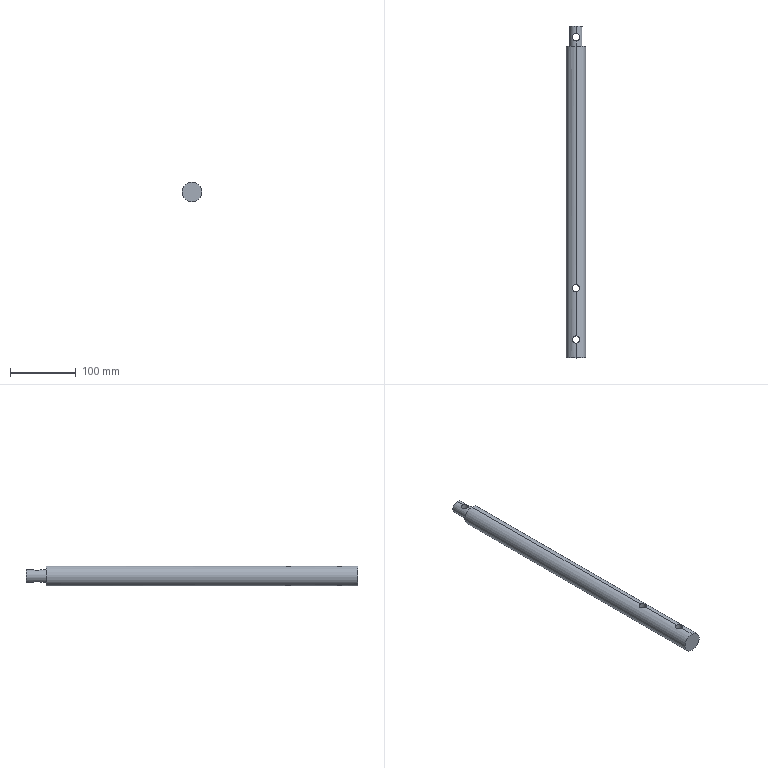Part | SolidWorks | features ICE 3, MoveFace 3, Extrusion 1 | 1 solid | 13 faces | box 30 x 504 x 30 mm | volume 335802 mm3 | cylinder 10 | plane 3 | commonest cylinder face diameters 11 x6 19 x2 30 x2
STEP:
#1=CARTESIAN_POINT('',(-5.5,288.,-13.955));
#2=VERTEX_POINT('',#1);
#3=CARTESIAN_POINT('',(0.,282.5,-15.));
#4=VERTEX_POINT('',#3);
#5=CARTESIAN_POINT('',(-5.5,288.,-13.955));
#6=CARTESIAN_POINT('',(-5.5,287.638,-13.955));
#7=CARTESIAN_POINT('',(-5.463,287.27,-13.97));
#8=CARTESIAN_POINT('',(-5.321,286.562,-14.025));
#9=CARTESIAN_POINT('',(-5.216,286.218,-14.065));
#10=CARTESIAN_POINT('',(-4.936,285.548,-14.165));
#11=CARTESIAN_POINT('',(-4.766,285.232,-14.224));
#12=CARTESIAN_POINT('',(-4.369,284.64,-14.351));
#13=CARTESIAN_POINT('',(-4.139,284.36,-14.42));
#14=CARTESIAN_POINT('',(-3.634,283.856,-14.555));
#15=CARTESIAN_POINT('',(-3.36,283.631,-14.622));
#16=CARTESIAN_POINT('',(-2.765,283.232,-14.746));
#17=CARTESIAN_POINT('',(-2.444,283.06,-14.803));
#18=CARTESIAN_POINT('',(-1.783,282.785,-14.897));
#19=CARTESIAN_POINT('',(-1.439,282.679,-14.935));
#20=CARTESIAN_POINT('',(-0.9036,282.572,-14.974));
#21=CARTESIAN_POINT('',(-0.7221,282.545,-14.984));
#22=CARTESIAN_POINT('',(-0.3611,282.509,-14.997));
#23=CARTESIAN_POINT('',(-0.1806,282.5,-15.));
#24=CARTESIAN_POINT('',(0.,282.5,-15.));
#25=B_SPLINE_CURVE_WITH_KNOTS('',3,(#5,#6,#7,#8,#9,#10,#11,#12,#13,#14,#15,#16,#17,#18,#19,#20,#21,#22,#23,#24),.UNSPECIFIED.,.F.,.F.,(4,2,2,2,2,2,2,2,2,4),(0.008677,0.009761,0.01084,0.01193,0.01301,0.0141,0.01518,0.01626,0.01681,0.01735),.UNSPECIFIED.);
#26=EDGE_CURVE('',#2,#4,#25,.T.);
#27=ORIENTED_EDGE('',*,*,#26,.F.);
#28=CARTESIAN_POINT('',(-5.5,288.,13.955));
#29=VERTEX_POINT('',#28);
#30=CARTESIAN_POINT('',(-5.5,288.,-215.));
#31=DIRECTION('',(0.,0.,1.));
#32=VECTOR('',#31,1000.);
#33=LINE('',#30,#32);
#34=EDGE_CURVE('',#2,#29,#33,.T.);
#35=ORIENTED_EDGE('',*,*,#34,.T.);
#36=CARTESIAN_POINT('',(0.,282.5,15.));
#37=VERTEX_POINT('',#36);
#38=CARTESIAN_POINT('',(0.,282.5,15.));
#39=CARTESIAN_POINT('',(-0.3624,282.5,15.));
#40=CARTESIAN_POINT('',(-0.7302,282.537,14.986));
#41=CARTESIAN_POINT('',(-1.438,282.679,14.935));
#42=CARTESIAN_POINT('',(-1.783,282.784,14.898));
#43=CARTESIAN_POINT('',(-2.453,283.064,14.802));
#44=CARTESIAN_POINT('',(-2.769,283.234,14.745));
#45=CARTESIAN_POINT('',(-3.361,283.632,14.622));
#46=CARTESIAN_POINT('',(-3.641,283.862,14.554));
#47=CARTESIAN_POINT('',(-4.145,284.368,14.418));
#48=CARTESIAN_POINT('',(-4.371,284.642,14.351));
#49=CARTESIAN_POINT('',(-4.768,285.236,14.223));
#50=CARTESIAN_POINT('',(-4.941,285.557,14.164));
#51=CARTESIAN_POINT('',(-5.216,286.218,14.065));
#52=CARTESIAN_POINT('',(-5.321,286.561,14.025));
#53=CARTESIAN_POINT('',(-5.428,287.096,13.983));
#54=CARTESIAN_POINT('',(-5.455,287.278,13.973));
#55=CARTESIAN_POINT('',(-5.491,287.639,13.959));
#56=CARTESIAN_POINT('',(-5.5,287.819,13.955));
#57=CARTESIAN_POINT('',(-5.5,288.,13.955));
#58=B_SPLINE_CURVE_WITH_KNOTS('',3,(#38,#39,#40,#41,#42,#43,#44,#45,#46,#47,#48,#49,#50,#51,#52,#53,#54,#55,#56,#57),.UNSPECIFIED.,.F.,.F.,(4,2,2,2,2,2,2,2,2,4),(0.008676,0.00976,0.01084,0.01193,0.01301,0.0141,0.01518,0.01626,0.01681,0.01735),.UNSPECIFIED.);
#59=EDGE_CURVE('',#37,#29,#58,.T.);
#60=ORIENTED_EDGE('',*,*,#59,.F.);
#61=CARTESIAN_POINT('',(5.5,288.,13.955));
#62=VERTEX_POINT('',#61);
#63=CARTESIAN_POINT('',(5.5,288.,13.955));
#64=CARTESIAN_POINT('',(5.5,287.633,13.955));
#65=CARTESIAN_POINT('',(5.464,287.273,13.97));
#66=CARTESIAN_POINT('',(5.322,286.565,14.024));
#67=CARTESIAN_POINT('',(5.215,286.214,14.065));
#68=CARTESIAN_POINT('',(4.937,285.55,14.165));
#69=CARTESIAN_POINT('',(4.768,285.235,14.224));
#70=CARTESIAN_POINT('',(4.469,284.789,14.319));
#71=CARTESIAN_POINT('',(4.361,284.644,14.353));
#72=CARTESIAN_POINT('',(4.133,284.367,14.42));
#73=CARTESIAN_POINT('',(4.013,284.235,14.454));
#74=CARTESIAN_POINT('',(3.636,283.858,14.555));
#75=CARTESIAN_POINT('',(3.361,283.631,14.622));
#76=CARTESIAN_POINT('',(2.761,283.229,14.747));
#77=CARTESIAN_POINT('',(2.445,283.061,14.803));
#78=CARTESIAN_POINT('',(1.949,282.854,14.874));
#79=CARTESIAN_POINT('',(1.78,282.793,14.895));
#80=CARTESIAN_POINT('',(1.434,282.687,14.932));
#81=CARTESIAN_POINT('',(1.256,282.642,14.948));
#82=CARTESIAN_POINT('',(0.7219,282.536,14.987));
#83=CARTESIAN_POINT('',(0.3626,282.5,15.));
#84=CARTESIAN_POINT('',(0.,282.5,15.));
#85=B_SPLINE_CURVE_WITH_KNOTS('',3,(#63,#64,#65,#66,#67,#68,#69,#70,#71,#72,#73,#74,#75,#76,#77,#78,#79,#80,#81,#82,#83,#84),.UNSPECIFIED.,.F.,.F.,(4,2,2,2,2,2,2,2,2,2,4),(0.,0.001085,0.002169,0.003254,0.003796,0.004338,0.005423,0.006507,0.00705,0.007592,0.008676),.UNSPECIFIED.);
#86=EDGE_CURVE('',#62,#37,#85,.T.);
#87=ORIENTED_EDGE('',*,*,#86,.F.);
#88=CARTESIAN_POINT('',(5.5,288.,-13.955));
#89=VERTEX_POINT('',#88);
#90=CARTESIAN_POINT('',(5.5,288.,-215.));
#91=DIRECTION('',(0.,0.,1.));
#92=VECTOR('',#91,1000.);
#93=LINE('',#90,#92);
#94=EDGE_CURVE('',#89,#62,#93,.T.);
#95=ORIENTED_EDGE('',*,*,#94,.F.);
#96=CARTESIAN_POINT('',(0.,282.5,-15.));
#97=CARTESIAN_POINT('',(0.1806,282.5,-15.));
#98=CARTESIAN_POINT('',(0.3612,282.509,-14.997));
#99=CARTESIAN_POINT('',(0.7226,282.545,-14.984));
#100=CARTESIAN_POINT('',(0.9044,282.572,-14.974));
#101=CARTESIAN_POINT('',(1.439,282.679,-14.935));
#102=CARTESIAN_POINT('',(1.783,282.785,-14.897));
#103=CARTESIAN_POINT('',(2.448,283.062,-14.803));
#104=CARTESIAN_POINT('',(2.769,283.234,-14.745));
#105=CARTESIAN_POINT('',(3.361,283.632,-14.622));
#106=CARTESIAN_POINT('',(3.637,283.858,-14.555));
#107=CARTESIAN_POINT('',(4.145,284.367,-14.418));
#108=CARTESIAN_POINT('',(4.371,284.643,-14.35));
#109=CARTESIAN_POINT('',(4.668,285.086,-14.255));
#110=CARTESIAN_POINT('',(4.76,285.239,-14.225));
#111=CARTESIAN_POINT('',(4.93,285.555,-14.167));
#112=CARTESIAN_POINT('',(5.008,285.72,-14.139));
#113=CARTESIAN_POINT('',(5.216,286.219,-14.065));
#114=CARTESIAN_POINT('',(5.321,286.563,-14.025));
#115=CARTESIAN_POINT('',(5.463,287.27,-13.97));
#116=CARTESIAN_POINT('',(5.5,287.638,-13.955));
#117=CARTESIAN_POINT('',(5.5,288.,-13.955));
#118=B_SPLINE_CURVE_WITH_KNOTS('',3,(#96,#97,#98,#99,#100,#101,#102,#103,#104,#105,#106,#107,#108,#109,#110,#111,#112,#113,#114,#115,#116,#117),.UNSPECIFIED.,.F.,.F.,(4,2,2,2,2,2,2,2,2,2,4),(0.01735,0.01789,0.01843,0.01952,0.0206,0.02168,0.02277,0.02331,0.02385,0.02493,0.02602),.UNSPECIFIED.);
#119=EDGE_CURVE('',#4,#89,#118,.T.);
#120=ORIENTED_EDGE('',*,*,#119,.F.);
#121=EDGE_LOOP('',(#27,#35,#60,#87,#95,#120));
#122=FACE_OUTER_BOUND('',#121,.T.);
#123=CARTESIAN_POINT('',(0.,288.,-215.));
#124=DIRECTION('',(0.,0.,1.));
#125=DIRECTION('',(1.,0.,0.));
#126=AXIS2_PLACEMENT_3D('',#123,#124,#125);
#127=CYLINDRICAL_SURFACE('',#126,5.5);
#128=ADVANCED_FACE('',(#122),#127,.F.);
#129=CARTESIAN_POINT('',(-5.5,210.,-13.955));
#130=VERTEX_POINT('',#129);
#131=CARTESIAN_POINT('',(0.,204.5,-15.));
#132=VERTEX_POINT('',#131);
#133=CARTESIAN_POINT('',(-5.5,210.,-13.955));
#134=CARTESIAN_POINT('',(-5.5,209.818,-13.955));
#135=CARTESIAN_POINT('',(-5.491,209.634,-13.959));
#136=CARTESIAN_POINT('',(-5.455,209.272,-13.973));
#137=CARTESIAN_POINT('',(-5.428,209.093,-13.984));
#138=CARTESIAN_POINT('',(-5.321,208.562,-14.025));
#139=CARTESIAN_POINT('',(-5.215,208.214,-14.065));
#140=CARTESIAN_POINT('',(-4.936,207.547,-14.165));
#141=CARTESIAN_POINT('',(-4.766,207.232,-14.224));
#142=CARTESIAN_POINT('',(-4.368,206.639,-14.352));
#143=CARTESIAN_POINT('',(-4.137,206.358,-14.421));
#144=CARTESIAN_POINT('',(-3.633,205.855,-14.556));
#145=CARTESIAN_POINT('',(-3.358,205.63,-14.622));
#146=CARTESIAN_POINT('',(-2.91,205.33,-14.716));
#147=CARTESIAN_POINT('',(-2.755,205.236,-14.746));
#148=CARTESIAN_POINT('',(-2.438,205.067,-14.801));
#149=CARTESIAN_POINT('',(-2.277,204.99,-14.827));
#150=CARTESIAN_POINT('',(-1.782,204.785,-14.897));
#151=CARTESIAN_POINT('',(-1.44,204.679,-14.935));
#152=CARTESIAN_POINT('',(-0.904,204.572,-14.974));
#153=CARTESIAN_POINT('',(-0.7225,204.545,-14.984));
#154=CARTESIAN_POINT('',(-0.3614,204.509,-14.997));
#155=CARTESIAN_POINT('',(-0.1808,204.5,-15.));
#156=CARTESIAN_POINT('',(0.,204.5,-15.));
#157=B_SPLINE_CURVE_WITH_KNOTS('',3,(#133,#134,#135,#136,#137,#138,#139,#140,#141,#142,#143,#144,#145,#146,#147,#148,#149,#150,#151,#152,#153,#154,#155,#156),.UNSPECIFIED.,.F.,.F.,(4,2,2,2,2,2,2,2,2,2,2,4),(0.02696,0.02751,0.02805,0.02913,0.03022,0.0313,0.03239,0.03293,0.03347,0.03456,0.0351,0.03564),.UNSPECIFIED.);
#158=EDGE_CURVE('',#130,#132,#157,.T.);
#159=ORIENTED_EDGE('',*,*,#158,.F.);
#160=CARTESIAN_POINT('',(-5.5,210.,13.955));
#161=VERTEX_POINT('',#160);
#162=CARTESIAN_POINT('',(-5.5,210.,-240.));
#163=DIRECTION('',(0.,0.,1.));
#164=VECTOR('',#163,1000.);
#165=LINE('',#162,#164);
#166=EDGE_CURVE('',#130,#161,#165,.T.);
#167=ORIENTED_EDGE('',*,*,#166,.T.);
#168=CARTESIAN_POINT('',(0.,204.5,15.));
#169=VERTEX_POINT('',#168);
#170=CARTESIAN_POINT('',(0.,204.5,15.));
#171=CARTESIAN_POINT('',(-0.182,204.5,15.));
#172=CARTESIAN_POINT('',(-0.3661,204.509,14.997));
#173=CARTESIAN_POINT('',(-0.7283,204.545,14.983));
#174=CARTESIAN_POINT('',(-0.9072,204.572,14.974));
#175=CARTESIAN_POINT('',(-1.438,204.679,14.935));
#176=CARTESIAN_POINT('',(-1.786,204.785,14.897));
#177=CARTESIAN_POINT('',(-2.454,205.065,14.802));
#178=CARTESIAN_POINT('',(-2.769,205.235,14.745));
#179=CARTESIAN_POINT('',(-3.363,205.633,14.621));
#180=CARTESIAN_POINT('',(-3.643,205.864,14.553));
#181=CARTESIAN_POINT('',(-4.146,206.369,14.418));
#182=CARTESIAN_POINT('',(-4.372,206.643,14.35));
#183=CARTESIAN_POINT('',(-4.671,207.091,14.254));
#184=CARTESIAN_POINT('',(-4.765,207.247,14.223));
#185=CARTESIAN_POINT('',(-4.934,207.563,14.166));
#186=CARTESIAN_POINT('',(-5.01,207.724,14.139));
#187=CARTESIAN_POINT('',(-5.216,208.218,14.065));
#188=CARTESIAN_POINT('',(-5.321,208.561,14.025));
#189=CARTESIAN_POINT('',(-5.428,209.096,13.983));
#190=CARTESIAN_POINT('',(-5.455,209.277,13.973));
#191=CARTESIAN_POINT('',(-5.491,209.639,13.959));
#192=CARTESIAN_POINT('',(-5.5,209.819,13.955));
#193=CARTESIAN_POINT('',(-5.5,210.,13.955));
#194=B_SPLINE_CURVE_WITH_KNOTS('',3,(#170,#171,#172,#173,#174,#175,#176,#177,#178,#179,#180,#181,#182,#183,#184,#185,#186,#187,#188,#189,#190,#191,#192,#193),.UNSPECIFIED.,.F.,.F.,(4,2,2,2,2,2,2,2,2,2,2,4),(0.02696,0.0275,0.02804,0.02912,0.03021,0.03129,0.03238,0.03292,0.03346,0.03455,0.03509,0.03563),.UNSPECIFIED.);
#195=EDGE_CURVE('',#169,#161,#194,.T.);
#196=ORIENTED_EDGE('',*,*,#195,.F.);
#197=CARTESIAN_POINT('',(5.5,210.,13.955));
#198=VERTEX_POINT('',#197);
#199=CARTESIAN_POINT('',(5.5,210.,13.955));
#200=CARTESIAN_POINT('',(5.5,209.634,13.955));
#201=CARTESIAN_POINT('',(5.464,209.275,13.97));
#202=CARTESIAN_POINT('',(5.322,208.566,14.024));
#203=CARTESIAN_POINT('',(5.214,208.214,14.065));
#204=CARTESIAN_POINT('',(4.938,207.551,14.165));
#205=CARTESIAN_POINT('',(4.769,207.236,14.223));
#206=CARTESIAN_POINT('',(4.368,206.638,14.352));
#207=CARTESIAN_POINT('',(4.14,206.361,14.42));
#208=CARTESIAN_POINT('',(3.763,205.984,14.521));
#209=CARTESIAN_POINT('',(3.631,205.865,14.555));
#210=CARTESIAN_POINT('',(3.354,205.638,14.621));
#211=CARTESIAN_POINT('',(3.209,205.529,14.654));
#212=CARTESIAN_POINT('',(2.761,205.23,14.747));
#213=CARTESIAN_POINT('',(2.447,205.061,14.803));
#214=CARTESIAN_POINT('',(1.784,204.785,14.897));
#215=CARTESIAN_POINT('',(1.432,204.677,14.936));
#216=CARTESIAN_POINT('',(0.7232,204.536,14.987));
#217=CARTESIAN_POINT('',(0.364,204.5,15.));
#218=CARTESIAN_POINT('',(0.,204.5,15.));
#219=B_SPLINE_CURVE_WITH_KNOTS('',3,(#199,#200,#201,#202,#203,#204,#205,#206,#207,#208,#209,#210,#211,#212,#213,#214,#215,#216,#217,#218),.UNSPECIFIED.,.F.,.F.,(4,2,2,2,2,2,2,2,2,4),(0.01828,0.01936,0.02045,0.02153,0.02262,0.02316,0.0237,0.02479,0.02587,0.02696),.UNSPECIFIED.);
#220=EDGE_CURVE('',#198,#169,#219,.T.);
#221=ORIENTED_EDGE('',*,*,#220,.F.);
#222=CARTESIAN_POINT('',(5.5,210.,-13.955));
#223=VERTEX_POINT('',#222);
#224=CARTESIAN_POINT('',(5.5,210.,-240.));
#225=DIRECTION('',(0.,0.,1.));
#226=VECTOR('',#225,1000.);
#227=LINE('',#224,#226);
#228=EDGE_CURVE('',#223,#198,#227,.T.);
#229=ORIENTED_EDGE('',*,*,#228,.F.);
#230=CARTESIAN_POINT('',(0.,204.5,-15.));
#231=CARTESIAN_POINT('',(0.1807,204.5,-15.));
#232=CARTESIAN_POINT('',(0.3616,204.509,-14.997));
#233=CARTESIAN_POINT('',(0.7235,204.545,-14.984));
#234=CARTESIAN_POINT('',(0.9054,204.572,-14.974));
#235=CARTESIAN_POINT('',(1.439,204.679,-14.935));
#236=CARTESIAN_POINT('',(1.783,204.785,-14.897));
#237=CARTESIAN_POINT('',(2.448,205.062,-14.803));
#238=CARTESIAN_POINT('',(2.769,205.235,-14.745));
#239=CARTESIAN_POINT('',(3.361,205.632,-14.622));
#240=CARTESIAN_POINT('',(3.637,205.858,-14.555));
#241=CARTESIAN_POINT('',(4.145,206.368,-14.418));
#242=CARTESIAN_POINT('',(4.371,206.643,-14.35));
#243=CARTESIAN_POINT('',(4.668,207.086,-14.255));
#244=CARTESIAN_POINT('',(4.76,207.239,-14.225));
#245=CARTESIAN_POINT('',(4.93,207.556,-14.167));
#246=CARTESIAN_POINT('',(5.009,207.72,-14.139));
#247=CARTESIAN_POINT('',(5.216,208.219,-14.065));
#248=CARTESIAN_POINT('',(5.321,208.562,-14.025));
#249=CARTESIAN_POINT('',(5.463,209.27,-13.97));
#250=CARTESIAN_POINT('',(5.5,209.638,-13.955));
#251=CARTESIAN_POINT('',(5.5,210.,-13.955));
#252=B_SPLINE_CURVE_WITH_KNOTS('',3,(#230,#231,#232,#233,#234,#235,#236,#237,#238,#239,#240,#241,#242,#243,#244,#245,#246,#247,#248,#249,#250,#251),.UNSPECIFIED.,.F.,.F.,(4,2,2,2,2,2,2,2,2,2,4),(0.0009354,0.001478,0.00202,0.003104,0.004189,0.005273,0.006357,0.006899,0.007442,0.008526,0.00961),.UNSPECIFIED.);
#253=EDGE_CURVE('',#132,#223,#252,.T.);
#254=ORIENTED_EDGE('',*,*,#253,.F.);
#255=EDGE_LOOP('',(#159,#167,#196,#221,#229,#254));
#256=FACE_OUTER_BOUND('',#255,.T.);
#257=CARTESIAN_POINT('',(0.,210.,-240.));
#258=DIRECTION('',(0.,0.,1.));
#259=DIRECTION('',(1.,0.,0.));
#260=AXIS2_PLACEMENT_3D('',#257,#258,#259);
#261=CYLINDRICAL_SURFACE('',#260,5.5);
#262=ADVANCED_FACE('',(#256),#261,.F.);
#263=CARTESIAN_POINT('',(-5.5,669.,-7.746));
#264=VERTEX_POINT('',#263);
#265=CARTESIAN_POINT('',(0.,663.5,-9.5));
#266=VERTEX_POINT('',#265);
#267=CARTESIAN_POINT('',(-5.5,669.,-7.746));
#268=CARTESIAN_POINT('',(-5.5,668.631,-7.746));
#269=CARTESIAN_POINT('',(-5.463,668.267,-7.772));
#270=CARTESIAN_POINT('',(-5.354,667.728,-7.848));
#271=CARTESIAN_POINT('',(-5.308,667.549,-7.879));
#272=CARTESIAN_POINT('',(-5.201,667.203,-7.95));
#273=CARTESIAN_POINT('',(-5.14,667.034,-7.99));
#274=CARTESIAN_POINT('',(-4.932,666.54,-8.121));
#275=CARTESIAN_POINT('',(-4.761,666.223,-8.224));
#276=CARTESIAN_POINT('',(-4.367,665.638,-8.44));
#277=CARTESIAN_POINT('',(-4.145,665.368,-8.552));
#278=CARTESIAN_POINT('',(-3.647,664.868,-8.776));
#279=CARTESIAN_POINT('',(-3.373,664.642,-8.886));
#280=CARTESIAN_POINT('',(-2.79,664.247,-9.086));
#281=CARTESIAN_POINT('',(-2.478,664.076,-9.178));
#282=CARTESIAN_POINT('',(-1.808,663.793,-9.333));
#283=CARTESIAN_POINT('',(-1.461,663.685,-9.394));
#284=CARTESIAN_POINT('',(-0.7448,663.538,-9.478));
#285=CARTESIAN_POINT('',(-0.3711,663.5,-9.5));
#286=CARTESIAN_POINT('',(0.,663.5,-9.5));
#287=B_SPLINE_CURVE_WITH_KNOTS('',3,(#267,#268,#269,#270,#271,#272,#273,#274,#275,#276,#277,#278,#279,#280,#281,#282,#283,#284,#285,#286),.UNSPECIFIED.,.F.,.F.,(4,2,2,2,2,2,2,2,2,4),(0.02644,0.02754,0.02809,0.02863,0.02973,0.03083,0.03193,0.03303,0.03412,0.03522),.UNSPECIFIED.);
#288=EDGE_CURVE('',#264,#266,#287,.T.);
#289=ORIENTED_EDGE('',*,*,#288,.F.);
#290=CARTESIAN_POINT('',(-5.5,669.,7.746));
#291=VERTEX_POINT('',#290);
#292=CARTESIAN_POINT('',(-5.5,669.,-240.));
#293=DIRECTION('',(0.,0.,1.));
#294=VECTOR('',#293,1000.);
#295=LINE('',#292,#294);
#296=EDGE_CURVE('',#264,#291,#295,.T.);
#297=ORIENTED_EDGE('',*,*,#296,.T.);
#298=CARTESIAN_POINT('',(0.,663.5,9.5));
#299=VERTEX_POINT('',#298);
#300=CARTESIAN_POINT('',(0.,663.5,9.5));
#301=CARTESIAN_POINT('',(-0.1849,663.5,9.5));
#302=CARTESIAN_POINT('',(-0.3717,663.509,9.494));
#303=CARTESIAN_POINT('',(-0.7383,663.547,9.473));
#304=CARTESIAN_POINT('',(-0.9193,663.574,9.457));
#305=CARTESIAN_POINT('',(-1.277,663.647,9.416));
#306=CARTESIAN_POINT('',(-1.454,663.692,9.39));
#307=CARTESIAN_POINT('',(-1.803,663.801,9.329));
#308=CARTESIAN_POINT('',(-1.975,663.864,9.294));
#309=CARTESIAN_POINT('',(-2.474,664.074,9.179));
#310=CARTESIAN_POINT('',(-2.787,664.245,9.087));
#311=CARTESIAN_POINT('',(-3.377,664.644,8.885));
#312=CARTESIAN_POINT('',(-3.65,664.871,8.775));
#313=CARTESIAN_POINT('',(-4.021,665.244,8.608));
#314=CARTESIAN_POINT('',(-4.139,665.374,8.552));
#315=CARTESIAN_POINT('',(-4.362,665.646,8.44));
#316=CARTESIAN_POINT('',(-4.468,665.788,8.384));
#317=CARTESIAN_POINT('',(-4.764,666.229,8.222));
#318=CARTESIAN_POINT('',(-4.932,666.539,8.121));
#319=CARTESIAN_POINT('',(-5.139,667.031,7.991));
#320=CARTESIAN_POINT('',(-5.2,667.2,7.951));
#321=CARTESIAN_POINT('',(-5.308,667.547,7.879));
#322=CARTESIAN_POINT('',(-5.353,667.726,7.848));
#323=CARTESIAN_POINT('',(-5.463,668.263,7.773));
#324=CARTESIAN_POINT('',(-5.5,668.628,7.746));
#325=CARTESIAN_POINT('',(-5.5,669.,7.746));
#326=B_SPLINE_CURVE_WITH_KNOTS('',3,(#300,#301,#302,#303,#304,#305,#306,#307,#308,#309,#310,#311,#312,#313,#314,#315,#316,#317,#318,#319,#320,#321,#322,#323,#324,#325),.UNSPECIFIED.,.F.,.F.,(4,2,2,2,2,2,2,2,2,2,2,2,4),(0.02631,0.02686,0.02741,0.02796,0.02851,0.02961,0.0307,0.03125,0.0318,0.0329,0.03345,0.03399,0.03509),.UNSPECIFIED.);
#327=EDGE_CURVE('',#299,#291,#326,.T.);
#328=ORIENTED_EDGE('',*,*,#327,.F.);
#329=CARTESIAN_POINT('',(5.5,669.,7.746));
#330=VERTEX_POINT('',#329);
#331=CARTESIAN_POINT('',(5.5,669.,7.746));
#332=CARTESIAN_POINT('',(5.5,668.815,7.746));
#333=CARTESIAN_POINT('',(5.49,668.628,7.753));
#334=CARTESIAN_POINT('',(5.453,668.261,7.779));
#335=CARTESIAN_POINT('',(5.426,668.081,7.798));
#336=CARTESIAN_POINT('',(5.317,667.545,7.874));
#337=CARTESIAN_POINT('',(5.207,667.193,7.947));
#338=CARTESIAN_POINT('',(4.929,666.533,8.123));
#339=CARTESIAN_POINT('',(4.759,666.221,8.225));
#340=CARTESIAN_POINT('',(4.362,665.631,8.443));
#341=CARTESIAN_POINT('',(4.138,665.36,8.556));
#342=CARTESIAN_POINT('',(3.767,664.988,8.722));
#343=CARTESIAN_POINT('',(3.636,664.87,8.778));
#344=CARTESIAN_POINT('',(3.363,664.644,8.886));
#345=CARTESIAN_POINT('',(3.22,664.537,8.939));
#346=CARTESIAN_POINT('',(2.778,664.24,9.09));
#347=CARTESIAN_POINT('',(2.467,664.071,9.18));
#348=CARTESIAN_POINT('',(1.805,663.792,9.333));
#349=CARTESIAN_POINT('',(1.45,663.682,9.396));
#350=CARTESIAN_POINT('',(0.7341,663.537,9.478));
#351=CARTESIAN_POINT('',(0.3703,663.5,9.5));
#352=CARTESIAN_POINT('',(0.,663.5,9.5));
#353=B_SPLINE_CURVE_WITH_KNOTS('',3,(#331,#332,#333,#334,#335,#336,#337,#338,#339,#340,#341,#342,#343,#344,#345,#346,#347,#348,#349,#350,#351,#352),.UNSPECIFIED.,.F.,.F.,(4,2,2,2,2,2,2,2,2,2,4),(0.01752,0.01807,0.01862,0.01972,0.02082,0.02192,0.02247,0.02302,0.02412,0.02522,0.02631),.UNSPECIFIED.);
#354=EDGE_CURVE('',#330,#299,#353,.T.);
#355=ORIENTED_EDGE('',*,*,#354,.F.);
#356=CARTESIAN_POINT('',(5.5,669.,-7.746));
#357=VERTEX_POINT('',#356);
#358=CARTESIAN_POINT('',(5.5,669.,-240.));
#359=DIRECTION('',(0.,0.,1.));
#360=VECTOR('',#359,1000.);
#361=LINE('',#358,#360);
#362=EDGE_CURVE('',#357,#330,#361,.T.);
#363=ORIENTED_EDGE('',*,*,#362,.F.);
#364=CARTESIAN_POINT('',(0.,663.5,-9.5));
#365=CARTESIAN_POINT('',(0.3722,663.5,-9.5));
#366=CARTESIAN_POINT('',(0.737,663.537,-9.478));
#367=CARTESIAN_POINT('',(1.453,663.683,-9.395));
#368=CARTESIAN_POINT('',(1.807,663.793,-9.333));
#369=CARTESIAN_POINT('',(2.47,664.073,-9.179));
#370=CARTESIAN_POINT('',(2.784,664.243,-9.088));
#371=CARTESIAN_POINT('',(3.377,664.644,-8.885));
#372=CARTESIAN_POINT('',(3.648,664.869,-8.776));
#373=CARTESIAN_POINT('',(4.143,665.365,-8.553));
#374=CARTESIAN_POINT('',(4.369,665.641,-8.439));
#375=CARTESIAN_POINT('',(4.762,666.226,-8.223));
#376=CARTESIAN_POINT('',(4.93,666.535,-8.122));
#377=CARTESIAN_POINT('',(5.207,667.193,-7.948));
#378=CARTESIAN_POINT('',(5.317,667.545,-7.873));
#379=CARTESIAN_POINT('',(5.462,668.26,-7.773));
#380=CARTESIAN_POINT('',(5.5,668.628,-7.746));
#381=CARTESIAN_POINT('',(5.5,669.,-7.746));
#382=B_SPLINE_CURVE_WITH_KNOTS('',3,(#364,#365,#366,#367,#368,#369,#370,#371,#372,#373,#374,#375,#376,#377,#378,#379,#380,#381),.UNSPECIFIED.,.F.,.F.,(4,2,2,2,2,2,2,2,4),(0.00003983,0.001141,0.002241,0.003342,0.004443,0.005544,0.006644,0.007745,0.008846),.UNSPECIFIED.);
#383=EDGE_CURVE('',#266,#357,#382,.T.);
#384=ORIENTED_EDGE('',*,*,#383,.F.);
#385=EDGE_LOOP('',(#289,#297,#328,#355,#363,#384));
#386=FACE_OUTER_BOUND('',#385,.T.);
#387=CARTESIAN_POINT('',(0.,669.,-240.));
#388=DIRECTION('',(0.,0.,1.));
#389=DIRECTION('',(1.,0.,0.));
#390=AXIS2_PLACEMENT_3D('',#387,#388,#389);
#391=CYLINDRICAL_SURFACE('',#390,5.5);
#392=ADVANCED_FACE('',(#386),#391,.F.);
#393=CARTESIAN_POINT('',(0.,686.,9.5));
#394=VERTEX_POINT('',#393);
#395=CARTESIAN_POINT('',(0.,686.,-9.5));
#396=VERTEX_POINT('',#395);
#397=CARTESIAN_POINT('',(0.,686.,0.));
#398=DIRECTION('',(0.,1.,0.));
#399=DIRECTION('',(0.,0.,1.));
#400=AXIS2_PLACEMENT_3D('',#397,#398,#399);
#401=CIRCLE('',#400,9.5);
#402=EDGE_CURVE('',#394,#396,#401,.T.);
#403=ORIENTED_EDGE('',*,*,#402,.F.);
#404=CARTESIAN_POINT('',(0.,674.5,9.5));
#405=VERTEX_POINT('',#404);
#406=CARTESIAN_POINT('',(0.,686.,9.5));
#407=DIRECTION('',(0.,-1.,0.));
#408=VECTOR('',#407,1000.);
#409=LINE('',#406,#408);
#410=EDGE_CURVE('',#394,#405,#409,.T.);
#411=ORIENTED_EDGE('',*,*,#410,.T.);
#412=CARTESIAN_POINT('',(0.,674.5,9.5));
#413=CARTESIAN_POINT('',(0.1843,674.5,9.5));
#414=CARTESIAN_POINT('',(0.3712,674.491,9.495));
#415=CARTESIAN_POINT('',(0.7387,674.453,9.473));
#416=CARTESIAN_POINT('',(0.92,674.426,9.457));
#417=CARTESIAN_POINT('',(1.278,674.353,9.415));
#418=CARTESIAN_POINT('',(1.454,674.307,9.39));
#419=CARTESIAN_POINT('',(1.802,674.2,9.329));
#420=CARTESIAN_POINT('',(1.975,674.136,9.294));
#421=CARTESIAN_POINT('',(2.475,673.925,9.178));
#422=CARTESIAN_POINT('',(2.788,673.754,9.087));
#423=CARTESIAN_POINT('',(3.23,673.456,8.936));
#424=CARTESIAN_POINT('',(3.373,673.348,8.882));
#425=CARTESIAN_POINT('',(3.645,673.123,8.774));
#426=CARTESIAN_POINT('',(3.775,673.004,8.719));
#427=CARTESIAN_POINT('',(4.145,672.631,8.552));
#428=CARTESIAN_POINT('',(4.369,672.36,8.439));
#429=CARTESIAN_POINT('',(4.765,671.77,8.222));
#430=CARTESIAN_POINT('',(4.932,671.46,8.121));
#431=CARTESIAN_POINT('',(5.139,670.968,7.99));
#432=CARTESIAN_POINT('',(5.2,670.8,7.95));
#433=CARTESIAN_POINT('',(5.307,670.454,7.879));
#434=CARTESIAN_POINT('',(5.353,670.275,7.848));
#435=CARTESIAN_POINT('',(5.463,669.736,7.773));
#436=CARTESIAN_POINT('',(5.5,669.371,7.746));
#437=CARTESIAN_POINT('',(5.5,669.,7.746));
#438=B_SPLINE_CURVE_WITH_KNOTS('',3,(#412,#413,#414,#415,#416,#417,#418,#419,#420,#421,#422,#423,#424,#425,#426,#427,#428,#429,#430,#431,#432,#433,#434,#435,#436,#437),.UNSPECIFIED.,.F.,.F.,(4,2,2,2,2,2,2,2,2,2,2,2,4),(0.008731,0.009281,0.00983,0.01038,0.01093,0.01203,0.01258,0.01313,0.01423,0.01533,0.01588,0.01643,0.01752),.UNSPECIFIED.);
#439=EDGE_CURVE('',#405,#330,#438,.T.);
#440=ORIENTED_EDGE('',*,*,#439,.T.);
#441=ORIENTED_EDGE('',*,*,#354,.T.);
#442=CARTESIAN_POINT('',(0.,655.,9.5));
#443=VERTEX_POINT('',#442);
#444=CARTESIAN_POINT('',(0.,686.,9.5));
#445=DIRECTION('',(0.,-1.,0.));
#446=VECTOR('',#445,1000.);
#447=LINE('',#444,#446);
#448=EDGE_CURVE('',#299,#443,#447,.T.);
#449=ORIENTED_EDGE('',*,*,#448,.T.);
#450=CARTESIAN_POINT('',(0.,655.,-9.5));
#451=VERTEX_POINT('',#450);
#452=CARTESIAN_POINT('',(0.,655.,0.));
#453=DIRECTION('',(0.,1.,0.));
#454=DIRECTION('',(0.,0.,1.));
#455=AXIS2_PLACEMENT_3D('',#452,#453,#454);
#456=CIRCLE('',#455,9.5);
#457=EDGE_CURVE('',#443,#451,#456,.T.);
#458=ORIENTED_EDGE('',*,*,#457,.T.);
#459=CARTESIAN_POINT('',(0.,686.,-9.5));
#460=DIRECTION('',(0.,-1.,0.));
#461=VECTOR('',#460,1000.);
#462=LINE('',#459,#461);
#463=EDGE_CURVE('',#266,#451,#462,.T.);
#464=ORIENTED_EDGE('',*,*,#463,.F.);
#465=ORIENTED_EDGE('',*,*,#383,.T.);
#466=CARTESIAN_POINT('',(0.,674.5,-9.5));
#467=VERTEX_POINT('',#466);
#468=CARTESIAN_POINT('',(5.5,669.,-7.746));
#469=CARTESIAN_POINT('',(5.5,669.372,-7.746));
#470=CARTESIAN_POINT('',(5.463,669.736,-7.773));
#471=CARTESIAN_POINT('',(5.354,670.274,-7.848));
#472=CARTESIAN_POINT('',(5.308,670.452,-7.879));
#473=CARTESIAN_POINT('',(5.2,670.8,-7.951));
#474=CARTESIAN_POINT('',(5.139,670.969,-7.991));
#475=CARTESIAN_POINT('',(4.93,671.464,-8.122));
#476=CARTESIAN_POINT('',(4.759,671.78,-8.225));
#477=CARTESIAN_POINT('',(4.364,672.366,-8.441));
#478=CARTESIAN_POINT('',(4.141,672.637,-8.554));
#479=CARTESIAN_POINT('',(3.644,673.135,-8.778));
#480=CARTESIAN_POINT('',(3.368,673.362,-8.888));
#481=CARTESIAN_POINT('',(2.783,673.757,-9.089));
#482=CARTESIAN_POINT('',(2.471,673.927,-9.179));
#483=CARTESIAN_POINT('',(1.97,674.138,-9.295));
#484=CARTESIAN_POINT('',(1.798,674.201,-9.33));
#485=CARTESIAN_POINT('',(1.45,674.309,-9.39));
#486=CARTESIAN_POINT('',(1.274,674.353,-9.416));
#487=CARTESIAN_POINT('',(0.7395,674.462,-9.478));
#488=CARTESIAN_POINT('',(0.3719,674.5,-9.5));
#489=CARTESIAN_POINT('',(0.,674.5,-9.5));
#490=B_SPLINE_CURVE_WITH_KNOTS('',3,(#468,#469,#470,#471,#472,#473,#474,#475,#476,#477,#478,#479,#480,#481,#482,#483,#484,#485,#486,#487,#488,#489),.UNSPECIFIED.,.F.,.F.,(4,2,2,2,2,2,2,2,2,2,4),(0.008846,0.009946,0.0105,0.01105,0.01215,0.01325,0.01435,0.01545,0.016,0.01655,0.01765),.UNSPECIFIED.);
#491=EDGE_CURVE('',#357,#467,#490,.T.);
#492=ORIENTED_EDGE('',*,*,#491,.T.);
#493=CARTESIAN_POINT('',(0.,686.,-9.5));
#494=DIRECTION('',(0.,-1.,0.));
#495=VECTOR('',#494,1000.);
#496=LINE('',#493,#495);
#497=EDGE_CURVE('',#396,#467,#496,.T.);
#498=ORIENTED_EDGE('',*,*,#497,.F.);
#499=EDGE_LOOP('',(#403,#411,#440,#441,#449,#458,#464,#465,#492,#498));
#500=FACE_OUTER_BOUND('',#499,.T.);
#501=CARTESIAN_POINT('',(0.,686.,0.));
#502=DIRECTION('',(0.,-1.,0.));
#503=DIRECTION('',(0.,0.,-1.));
#504=AXIS2_PLACEMENT_3D('',#501,#502,#503);
#505=CYLINDRICAL_SURFACE('',#504,9.5);
#506=ADVANCED_FACE('',(#500),#505,.T.);
#507=CARTESIAN_POINT('',(0.,655.,15.));
#508=VERTEX_POINT('',#507);
#509=CARTESIAN_POINT('',(0.,655.,-15.));
#510=VERTEX_POINT('',#509);
#511=CARTESIAN_POINT('',(0.,655.,0.));
#512=DIRECTION('',(0.,1.,0.));
#513=DIRECTION('',(0.,0.,1.));
#514=AXIS2_PLACEMENT_3D('',#511,#512,#513);
#515=CIRCLE('',#514,15.);
#516=EDGE_CURVE('',#508,#510,#515,.T.);
#517=ORIENTED_EDGE('',*,*,#516,.F.);
#518=CARTESIAN_POINT('',(0.,293.5,15.));
#519=VERTEX_POINT('',#518);
#520=CARTESIAN_POINT('',(0.,656.,15.));
#521=DIRECTION('',(0.,-1.,0.));
#522=VECTOR('',#521,1000.);
#523=LINE('',#520,#522);
#524=EDGE_CURVE('',#508,#519,#523,.T.);
#525=ORIENTED_EDGE('',*,*,#524,.T.);
#526=CARTESIAN_POINT('',(0.,293.5,15.));
#527=CARTESIAN_POINT('',(0.3625,293.5,15.));
#528=CARTESIAN_POINT('',(0.7223,293.465,14.987));
#529=CARTESIAN_POINT('',(1.258,293.357,14.948));
#530=CARTESIAN_POINT('',(1.435,293.312,14.932));
#531=CARTESIAN_POINT('',(1.781,293.207,14.895));
#532=CARTESIAN_POINT('',(1.951,293.146,14.874));
#533=CARTESIAN_POINT('',(2.282,293.007,14.826));
#534=CARTESIAN_POINT('',(2.444,292.93,14.8));
#535=CARTESIAN_POINT('',(2.761,292.76,14.745));
#536=CARTESIAN_POINT('',(2.917,292.666,14.714));
#537=CARTESIAN_POINT('',(3.364,292.366,14.621));
#538=CARTESIAN_POINT('',(3.639,292.14,14.554));
#539=CARTESIAN_POINT('',(4.143,291.635,14.419));
#540=CARTESIAN_POINT('',(4.373,291.355,14.35));
#541=CARTESIAN_POINT('',(4.769,290.762,14.223));
#542=CARTESIAN_POINT('',(4.938,290.448,14.165));
#543=CARTESIAN_POINT('',(5.147,289.948,14.09));
#544=CARTESIAN_POINT('',(5.209,289.776,14.067));
#545=CARTESIAN_POINT('',(5.314,289.43,14.027));
#546=CARTESIAN_POINT('',(5.358,289.256,14.011));
#547=CARTESIAN_POINT('',(5.464,288.727,13.97));
#548=CARTESIAN_POINT('',(5.5,288.367,13.955));
#549=CARTESIAN_POINT('',(5.5,288.,13.955));
#550=B_SPLINE_CURVE_WITH_KNOTS('',3,(#526,#527,#528,#529,#530,#531,#532,#533,#534,#535,#536,#537,#538,#539,#540,#541,#542,#543,#544,#545,#546,#547,#548,#549),.UNSPECIFIED.,.F.,.F.,(4,2,2,2,2,2,2,2,2,2,2,4),(0.02602,0.0271,0.02764,0.02819,0.02873,0.02927,0.03035,0.03144,0.03252,0.03306,0.03361,0.03469),.UNSPECIFIED.);
#551=EDGE_CURVE('',#519,#62,#550,.T.);
#552=ORIENTED_EDGE('',*,*,#551,.T.);
#553=ORIENTED_EDGE('',*,*,#86,.T.);
#554=CARTESIAN_POINT('',(0.,215.5,15.));
#555=VERTEX_POINT('',#554);
#556=CARTESIAN_POINT('',(0.,656.,15.));
#557=DIRECTION('',(0.,-1.,0.));
#558=VECTOR('',#557,1000.);
#559=LINE('',#556,#558);
#560=EDGE_CURVE('',#37,#555,#559,.T.);
#561=ORIENTED_EDGE('',*,*,#560,.T.);
#562=CARTESIAN_POINT('',(0.,215.5,15.));
#563=CARTESIAN_POINT('',(0.3621,215.5,15.));
#564=CARTESIAN_POINT('',(0.7219,215.465,14.987));
#565=CARTESIAN_POINT('',(1.258,215.357,14.948));
#566=CARTESIAN_POINT('',(1.435,215.313,14.932));
#567=CARTESIAN_POINT('',(1.781,215.207,14.895));
#568=CARTESIAN_POINT('',(1.95,215.146,14.874));
#569=CARTESIAN_POINT('',(2.281,215.008,14.826));
#570=CARTESIAN_POINT('',(2.443,214.931,14.801));
#571=CARTESIAN_POINT('',(2.76,214.76,14.745));
#572=CARTESIAN_POINT('',(2.916,214.667,14.715));
#573=CARTESIAN_POINT('',(3.363,214.367,14.621));
#574=CARTESIAN_POINT('',(3.637,214.141,14.555));
#575=CARTESIAN_POINT('',(4.142,213.636,14.419));
#576=CARTESIAN_POINT('',(4.372,213.356,14.35));
#577=CARTESIAN_POINT('',(4.768,212.764,14.223));
#578=CARTESIAN_POINT('',(4.937,212.45,14.165));
#579=CARTESIAN_POINT('',(5.146,211.949,14.09));
#580=CARTESIAN_POINT('',(5.208,211.778,14.067));
#581=CARTESIAN_POINT('',(5.313,211.433,14.028));
#582=CARTESIAN_POINT('',(5.401,211.084,13.994));
#583=CARTESIAN_POINT('',(5.455,210.727,13.973));
#584=CARTESIAN_POINT('',(5.491,210.366,13.959));
#585=CARTESIAN_POINT('',(5.5,210.183,13.955));
#586=CARTESIAN_POINT('',(5.5,210.,13.955));
#587=B_SPLINE_CURVE_WITH_KNOTS('',3,(#562,#563,#564,#565,#566,#567,#568,#569,#570,#571,#572,#573,#574,#575,#576,#577,#578,#579,#580,#581,#582,#583,#584,#585,#586),.UNSPECIFIED.,.F.,.F.,(4,2,2,2,2,2,2,2,2,2,1,2,4),(0.009602,0.01069,0.01123,0.01177,0.01231,0.01286,0.01394,0.01503,0.01611,0.01665,0.01719,0.01774,0.01828),.UNSPECIFIED.);
#588=EDGE_CURVE('',#555,#198,#587,.T.);
#589=ORIENTED_EDGE('',*,*,#588,.T.);
#590=ORIENTED_EDGE('',*,*,#220,.T.);
#591=CARTESIAN_POINT('',(0.,182.,15.));
#592=VERTEX_POINT('',#591);
#593=CARTESIAN_POINT('',(0.,656.,15.));
#594=DIRECTION('',(0.,-1.,0.));
#595=VECTOR('',#594,1000.);
#596=LINE('',#593,#595);
#597=EDGE_CURVE('',#169,#592,#596,.T.);
#598=ORIENTED_EDGE('',*,*,#597,.T.);
#599=CARTESIAN_POINT('',(0.,182.,-15.));
#600=VERTEX_POINT('',#599);
#601=CARTESIAN_POINT('',(0.,182.,0.));
#602=DIRECTION('',(0.,1.,0.));
#603=DIRECTION('',(0.,0.,1.));
#604=AXIS2_PLACEMENT_3D('',#601,#602,#603);
#605=CIRCLE('',#604,15.);
#606=EDGE_CURVE('',#592,#600,#605,.T.);
#607=ORIENTED_EDGE('',*,*,#606,.T.);
#608=CARTESIAN_POINT('',(0.,656.,-15.));
#609=DIRECTION('',(0.,-1.,0.));
#610=VECTOR('',#609,1000.);
#611=LINE('',#608,#610);
#612=EDGE_CURVE('',#132,#600,#611,.T.);
#613=ORIENTED_EDGE('',*,*,#612,.F.);
#614=ORIENTED_EDGE('',*,*,#253,.T.);
#615=CARTESIAN_POINT('',(0.,215.5,-15.));
#616=VERTEX_POINT('',#615);
#617=CARTESIAN_POINT('',(5.5,210.,-13.955));
#618=CARTESIAN_POINT('',(5.5,210.362,-13.955));
#619=CARTESIAN_POINT('',(5.465,210.722,-13.969));
#620=CARTESIAN_POINT('',(5.357,211.257,-14.011));
#621=CARTESIAN_POINT('',(5.313,211.435,-14.028));
#622=CARTESIAN_POINT('',(5.207,211.78,-14.067));
#623=CARTESIAN_POINT('',(5.146,211.949,-14.09));
#624=CARTESIAN_POINT('',(5.008,212.28,-14.139));
#625=CARTESIAN_POINT('',(4.931,212.442,-14.167));
#626=CARTESIAN_POINT('',(4.761,212.759,-14.225));
#627=CARTESIAN_POINT('',(4.668,212.915,-14.256));
#628=CARTESIAN_POINT('',(4.368,213.361,-14.351));
#629=CARTESIAN_POINT('',(4.142,213.636,-14.419));
#630=CARTESIAN_POINT('',(3.638,214.14,-14.554));
#631=CARTESIAN_POINT('',(3.358,214.371,-14.622));
#632=CARTESIAN_POINT('',(2.765,214.768,-14.746));
#633=CARTESIAN_POINT('',(2.451,214.937,-14.802));
#634=CARTESIAN_POINT('',(1.95,215.146,-14.874));
#635=CARTESIAN_POINT('',(1.778,215.208,-14.895));
#636=CARTESIAN_POINT('',(1.433,215.313,-14.932));
#637=CARTESIAN_POINT('',(1.084,215.401,-14.964));
#638=CARTESIAN_POINT('',(0.7269,215.455,-14.983));
#639=CARTESIAN_POINT('',(0.3661,215.491,-14.997));
#640=CARTESIAN_POINT('',(0.1827,215.5,-15.));
#641=CARTESIAN_POINT('',(0.,215.5,-15.));
#642=B_SPLINE_CURVE_WITH_KNOTS('',3,(#617,#618,#619,#620,#621,#622,#623,#624,#625,#626,#627,#628,#629,#630,#631,#632,#633,#634,#635,#636,#637,#638,#639,#640,#641),.UNSPECIFIED.,.F.,.F.,(4,2,2,2,2,2,2,2,2,2,1,2,4),(0.00961,0.01069,0.01124,0.01178,0.01232,0.01286,0.01395,0.01503,0.01612,0.01666,0.0172,0.01774,0.01829),.UNSPECIFIED.);
#643=EDGE_CURVE('',#223,#616,#642,.T.);
#644=ORIENTED_EDGE('',*,*,#643,.T.);
#645=CARTESIAN_POINT('',(0.,656.,-15.));
#646=DIRECTION('',(0.,-1.,0.));
#647=VECTOR('',#646,1000.);
#648=LINE('',#645,#647);
#649=EDGE_CURVE('',#4,#616,#648,.T.);
#650=ORIENTED_EDGE('',*,*,#649,.F.);
#651=ORIENTED_EDGE('',*,*,#119,.T.);
#652=CARTESIAN_POINT('',(0.,293.5,-15.));
#653=VERTEX_POINT('',#652);
#654=CARTESIAN_POINT('',(5.5,288.,-13.955));
#655=CARTESIAN_POINT('',(5.5,288.363,-13.955));
#656=CARTESIAN_POINT('',(5.465,288.722,-13.969));
#657=CARTESIAN_POINT('',(5.357,289.257,-14.011));
#658=CARTESIAN_POINT('',(5.313,289.435,-14.028));
#659=CARTESIAN_POINT('',(5.207,289.781,-14.067));
#660=CARTESIAN_POINT('',(5.146,289.95,-14.09));
#661=CARTESIAN_POINT('',(5.008,290.281,-14.14));
#662=CARTESIAN_POINT('',(4.931,290.443,-14.167));
#663=CARTESIAN_POINT('',(4.761,290.76,-14.225));
#664=CARTESIAN_POINT('',(4.667,290.915,-14.256));
#665=CARTESIAN_POINT('',(4.367,291.362,-14.352));
#666=CARTESIAN_POINT('',(4.141,291.637,-14.419));
#667=CARTESIAN_POINT('',(3.637,292.141,-14.555));
#668=CARTESIAN_POINT('',(3.356,292.372,-14.623));
#669=CARTESIAN_POINT('',(2.763,292.769,-14.746));
#670=CARTESIAN_POINT('',(2.449,292.938,-14.803));
#671=CARTESIAN_POINT('',(1.948,293.147,-14.874));
#672=CARTESIAN_POINT('',(1.776,293.208,-14.895));
#673=CARTESIAN_POINT('',(1.431,293.314,-14.933));
#674=CARTESIAN_POINT('',(1.256,293.358,-14.948));
#675=CARTESIAN_POINT('',(0.7268,293.464,-14.987));
#676=CARTESIAN_POINT('',(0.3669,293.5,-15.));
#677=CARTESIAN_POINT('',(0.,293.5,-15.));
#678=B_SPLINE_CURVE_WITH_KNOTS('',3,(#654,#655,#656,#657,#658,#659,#660,#661,#662,#663,#664,#665,#666,#667,#668,#669,#670,#671,#672,#673,#674,#675,#676,#677),.UNSPECIFIED.,.F.,.F.,(4,2,2,2,2,2,2,2,2,2,2,4),(0.02602,0.0271,0.02764,0.02819,0.02873,0.02927,0.03036,0.03144,0.03252,0.03307,0.03361,0.03469),.UNSPECIFIED.);
#679=EDGE_CURVE('',#89,#653,#678,.T.);
#680=ORIENTED_EDGE('',*,*,#679,.T.);
#681=CARTESIAN_POINT('',(0.,656.,-15.));
#682=DIRECTION('',(0.,-1.,0.));
#683=VECTOR('',#682,1000.);
#684=LINE('',#681,#683);
#685=EDGE_CURVE('',#510,#653,#684,.T.);
#686=ORIENTED_EDGE('',*,*,#685,.F.);
#687=EDGE_LOOP('',(#517,#525,#552,#553,#561,#589,#590,#598,#607,#613,#614,#644,#650,#651,#680,#686));
#688=FACE_OUTER_BOUND('',#687,.T.);
#689=CARTESIAN_POINT('',(0.,656.,0.));
#690=DIRECTION('',(0.,-1.,0.));
#691=DIRECTION('',(0.,0.,-1.));
#692=AXIS2_PLACEMENT_3D('',#689,#690,#691);
#693=CYLINDRICAL_SURFACE('',#692,15.);
#694=ADVANCED_FACE('',(#688),#693,.T.);
#695=ORIENTED_EDGE('',*,*,#524,.F.);
#696=CARTESIAN_POINT('',(0.,655.,0.));
#697=DIRECTION('',(0.,1.,0.));
#698=DIRECTION('',(0.,0.,1.));
#699=AXIS2_PLACEMENT_3D('',#696,#697,#698);
#700=CIRCLE('',#699,15.);
#701=EDGE_CURVE('',#510,#508,#700,.T.);
#702=ORIENTED_EDGE('',*,*,#701,.F.);
#703=ORIENTED_EDGE('',*,*,#685,.T.);
#704=CARTESIAN_POINT('',(0.,293.5,-15.));
#705=CARTESIAN_POINT('',(-0.367,293.5,-15.));
#706=CARTESIAN_POINT('',(-0.7272,293.464,-14.987));
#707=CARTESIAN_POINT('',(-1.435,293.322,-14.935));
#708=CARTESIAN_POINT('',(-1.786,293.214,-14.897));
#709=CARTESIAN_POINT('',(-2.451,292.937,-14.802));
#710=CARTESIAN_POINT('',(-2.766,292.767,-14.746));
#711=CARTESIAN_POINT('',(-3.213,292.468,-14.653));
#712=CARTESIAN_POINT('',(-3.358,292.36,-14.62));
#713=CARTESIAN_POINT('',(-3.635,292.132,-14.554));
#714=CARTESIAN_POINT('',(-3.767,292.012,-14.52));
#715=CARTESIAN_POINT('',(-4.143,291.634,-14.419));
#716=CARTESIAN_POINT('',(-4.37,291.359,-14.351));
#717=CARTESIAN_POINT('',(-4.771,290.759,-14.222));
#718=CARTESIAN_POINT('',(-4.94,290.444,-14.164));
#719=CARTESIAN_POINT('',(-5.146,289.949,-14.09));
#720=CARTESIAN_POINT('',(-5.207,289.78,-14.067));
#721=CARTESIAN_POINT('',(-5.313,289.433,-14.028));
#722=CARTESIAN_POINT('',(-5.358,289.256,-14.011));
#723=CARTESIAN_POINT('',(-5.465,288.722,-13.969));
#724=CARTESIAN_POINT('',(-5.5,288.363,-13.955));
#725=CARTESIAN_POINT('',(-5.5,288.,-13.955));
#726=B_SPLINE_CURVE_WITH_KNOTS('',3,(#704,#705,#706,#707,#708,#709,#710,#711,#712,#713,#714,#715,#716,#717,#718,#719,#720,#721,#722,#723,#724,#725),.UNSPECIFIED.,.F.,.F.,(4,2,2,2,2,2,2,2,2,2,4),(0.,0.001085,0.002169,0.003254,0.003796,0.004339,0.005423,0.006508,0.00705,0.007592,0.008677),.UNSPECIFIED.);
#727=EDGE_CURVE('',#653,#2,#726,.T.);
#728=ORIENTED_EDGE('',*,*,#727,.T.);
#729=ORIENTED_EDGE('',*,*,#26,.T.);
#730=ORIENTED_EDGE('',*,*,#649,.T.);
#731=CARTESIAN_POINT('',(0.,215.5,-15.));
#732=CARTESIAN_POINT('',(-0.3655,215.5,-15.));
#733=CARTESIAN_POINT('',(-0.7254,215.464,-14.987));
#734=CARTESIAN_POINT('',(-1.434,215.322,-14.935));
#735=CARTESIAN_POINT('',(-1.786,215.214,-14.897));
#736=CARTESIAN_POINT('',(-2.45,214.937,-14.802));
#737=CARTESIAN_POINT('',(-2.765,214.768,-14.746));
#738=CARTESIAN_POINT('',(-3.363,214.367,-14.621));
#739=CARTESIAN_POINT('',(-3.64,214.138,-14.554));
#740=CARTESIAN_POINT('',(-4.017,213.761,-14.453));
#741=CARTESIAN_POINT('',(-4.137,213.629,-14.419));
#742=CARTESIAN_POINT('',(-4.364,213.353,-14.352));
#743=CARTESIAN_POINT('',(-4.472,213.207,-14.318));
#744=CARTESIAN_POINT('',(-4.771,212.76,-14.223));
#745=CARTESIAN_POINT('',(-4.939,212.445,-14.164));
#746=CARTESIAN_POINT('',(-5.215,211.784,-14.065));
#747=CARTESIAN_POINT('',(-5.323,211.432,-14.024));
#748=CARTESIAN_POINT('',(-5.464,210.723,-13.97));
#749=CARTESIAN_POINT('',(-5.5,210.364,-13.955));
#750=CARTESIAN_POINT('',(-5.5,210.,-13.955));
#751=B_SPLINE_CURVE_WITH_KNOTS('',3,(#731,#732,#733,#734,#735,#736,#737,#738,#739,#740,#741,#742,#743,#744,#745,#746,#747,#748,#749,#750),.UNSPECIFIED.,.F.,.F.,(4,2,2,2,2,2,2,2,2,4),(0.01829,0.01937,0.02046,0.02154,0.02263,0.02317,0.02371,0.02479,0.02588,0.02696),.UNSPECIFIED.);
#752=EDGE_CURVE('',#616,#130,#751,.T.);
#753=ORIENTED_EDGE('',*,*,#752,.T.);
#754=ORIENTED_EDGE('',*,*,#158,.T.);
#755=ORIENTED_EDGE('',*,*,#612,.T.);
#756=CARTESIAN_POINT('',(0.,182.,0.));
#757=DIRECTION('',(0.,1.,0.));
#758=DIRECTION('',(0.,0.,1.));
#759=AXIS2_PLACEMENT_3D('',#756,#757,#758);
#760=CIRCLE('',#759,15.);
#761=EDGE_CURVE('',#600,#592,#760,.T.);
#762=ORIENTED_EDGE('',*,*,#761,.T.);
#763=ORIENTED_EDGE('',*,*,#597,.F.);
#764=ORIENTED_EDGE('',*,*,#195,.T.);
#765=CARTESIAN_POINT('',(-5.5,210.,13.955));
#766=CARTESIAN_POINT('',(-5.5,210.181,13.955));
#767=CARTESIAN_POINT('',(-5.491,210.362,13.959));
#768=CARTESIAN_POINT('',(-5.455,210.723,13.973));
#769=CARTESIAN_POINT('',(-5.428,210.905,13.983));
#770=CARTESIAN_POINT('',(-5.321,211.439,14.025));
#771=CARTESIAN_POINT('',(-5.215,211.783,14.065));
#772=CARTESIAN_POINT('',(-4.939,212.447,14.164));
#773=CARTESIAN_POINT('',(-4.766,212.768,14.224));
#774=CARTESIAN_POINT('',(-4.369,213.36,14.351));
#775=CARTESIAN_POINT('',(-4.143,213.635,14.419));
#776=CARTESIAN_POINT('',(-3.634,214.144,14.556));
#777=CARTESIAN_POINT('',(-3.359,214.37,14.622));
#778=CARTESIAN_POINT('',(-2.915,214.667,14.715));
#779=CARTESIAN_POINT('',(-2.762,214.76,14.744));
#780=CARTESIAN_POINT('',(-2.445,214.93,14.8));
#781=CARTESIAN_POINT('',(-2.281,215.008,14.827));
#782=CARTESIAN_POINT('',(-1.781,215.216,14.898));
#783=CARTESIAN_POINT('',(-1.438,215.321,14.935));
#784=CARTESIAN_POINT('',(-0.7301,215.463,14.986));
#785=CARTESIAN_POINT('',(-0.3621,215.5,15.));
#786=CARTESIAN_POINT('',(0.,215.5,15.));
#787=B_SPLINE_CURVE_WITH_KNOTS('',3,(#765,#766,#767,#768,#769,#770,#771,#772,#773,#774,#775,#776,#777,#778,#779,#780,#781,#782,#783,#784,#785,#786),.UNSPECIFIED.,.F.,.F.,(4,2,2,2,2,2,2,2,2,2,4),(0.0009274,0.00147,0.002012,0.003096,0.00418,0.005265,0.006349,0.006891,0.007434,0.008518,0.009602),.UNSPECIFIED.);
#788=EDGE_CURVE('',#161,#555,#787,.T.);
#789=ORIENTED_EDGE('',*,*,#788,.T.);
#790=ORIENTED_EDGE('',*,*,#560,.F.);
#791=ORIENTED_EDGE('',*,*,#59,.T.);
#792=CARTESIAN_POINT('',(-5.5,288.,13.955));
#793=CARTESIAN_POINT('',(-5.5,288.181,13.955));
#794=CARTESIAN_POINT('',(-5.491,288.361,13.959));
#795=CARTESIAN_POINT('',(-5.455,288.722,13.973));
#796=CARTESIAN_POINT('',(-5.428,288.904,13.983));
#797=CARTESIAN_POINT('',(-5.321,289.439,14.025));
#798=CARTESIAN_POINT('',(-5.215,289.783,14.065));
#799=CARTESIAN_POINT('',(-4.939,290.447,14.164));
#800=CARTESIAN_POINT('',(-4.766,290.767,14.224));
#801=CARTESIAN_POINT('',(-4.369,291.36,14.351));
#802=CARTESIAN_POINT('',(-4.143,291.635,14.419));
#803=CARTESIAN_POINT('',(-3.635,292.143,14.555));
#804=CARTESIAN_POINT('',(-3.359,292.37,14.622));
#805=CARTESIAN_POINT('',(-2.915,292.667,14.715));
#806=CARTESIAN_POINT('',(-2.762,292.759,14.744));
#807=CARTESIAN_POINT('',(-2.446,292.93,14.8));
#808=CARTESIAN_POINT('',(-2.281,293.008,14.826));
#809=CARTESIAN_POINT('',(-1.781,293.216,14.898));
#810=CARTESIAN_POINT('',(-1.438,293.321,14.935));
#811=CARTESIAN_POINT('',(-0.7304,293.463,14.986));
#812=CARTESIAN_POINT('',(-0.3623,293.5,15.));
#813=CARTESIAN_POINT('',(0.,293.5,15.));
#814=B_SPLINE_CURVE_WITH_KNOTS('',3,(#792,#793,#794,#795,#796,#797,#798,#799,#800,#801,#802,#803,#804,#805,#806,#807,#808,#809,#810,#811,#812,#813),.UNSPECIFIED.,.F.,.F.,(4,2,2,2,2,2,2,2,2,2,4),(0.01735,0.01789,0.01843,0.01951,0.0206,0.02168,0.02277,0.02331,0.02385,0.02493,0.02602),.UNSPECIFIED.);
#815=EDGE_CURVE('',#29,#519,#814,.T.);
#816=ORIENTED_EDGE('',*,*,#815,.T.);
#817=EDGE_LOOP('',(#695,#702,#703,#728,#729,#730,#753,#754,#755,#762,#763,#764,#789,#790,#791,#816));
#818=FACE_OUTER_BOUND('',#817,.T.);
#819=CARTESIAN_POINT('',(0.,656.,0.));
#820=DIRECTION('',(0.,-1.,0.));
#821=DIRECTION('',(0.,0.,-1.));
#822=AXIS2_PLACEMENT_3D('',#819,#820,#821);
#823=CYLINDRICAL_SURFACE('',#822,15.);
#824=ADVANCED_FACE('',(#818),#823,.T.);
#825=CARTESIAN_POINT('',(0.,655.,0.));
#826=DIRECTION('',(0.,1.,0.));
#827=DIRECTION('',(0.,0.,1.));
#828=AXIS2_PLACEMENT_3D('',#825,#826,#827);
#829=CIRCLE('',#828,9.5);
#830=EDGE_CURVE('',#451,#443,#829,.T.);
#831=ORIENTED_EDGE('',*,*,#830,.F.);
#832=ORIENTED_EDGE('',*,*,#457,.F.);
#833=EDGE_LOOP('',(#831,#832));
#834=FACE_BOUND('',#833,.T.);
#835=ORIENTED_EDGE('',*,*,#701,.T.);
#836=ORIENTED_EDGE('',*,*,#516,.T.);
#837=EDGE_LOOP('',(#835,#836));
#838=FACE_OUTER_BOUND('',#837,.T.);
#839=CARTESIAN_POINT('',(0.,655.,0.));
#840=DIRECTION('',(0.,1.,0.));
#841=DIRECTION('',(0.,0.,1.));
#842=AXIS2_PLACEMENT_3D('',#839,#840,#841);
#843=PLANE('',#842);
#844=ADVANCED_FACE('',(#834,#838),#843,.T.);
#845=ORIENTED_EDGE('',*,*,#761,.F.);
#846=ORIENTED_EDGE('',*,*,#606,.F.);
#847=EDGE_LOOP('',(#845,#846));
#848=FACE_OUTER_BOUND('',#847,.T.);
#849=CARTESIAN_POINT('',(0.,182.,0.));
#850=DIRECTION('',(0.,1.,0.));
#851=DIRECTION('',(0.,0.,1.));
#852=AXIS2_PLACEMENT_3D('',#849,#850,#851);
#853=PLANE('',#852);
#854=ADVANCED_FACE('',(#848),#853,.F.);
#855=ORIENTED_EDGE('',*,*,#410,.F.);
#856=CARTESIAN_POINT('',(0.,686.,0.));
#857=DIRECTION('',(0.,1.,0.));
#858=DIRECTION('',(0.,0.,1.));
#859=AXIS2_PLACEMENT_3D('',#856,#857,#858);
#860=CIRCLE('',#859,9.5);
#861=EDGE_CURVE('',#396,#394,#860,.T.);
#862=ORIENTED_EDGE('',*,*,#861,.F.);
#863=ORIENTED_EDGE('',*,*,#497,.T.);
#864=CARTESIAN_POINT('',(0.,674.5,-9.5));
#865=CARTESIAN_POINT('',(-0.3714,674.5,-9.5));
#866=CARTESIAN_POINT('',(-0.7361,674.463,-9.478));
#867=CARTESIAN_POINT('',(-1.453,674.317,-9.395));
#868=CARTESIAN_POINT('',(-1.807,674.207,-9.333));
#869=CARTESIAN_POINT('',(-2.47,673.927,-9.18));
#870=CARTESIAN_POINT('',(-2.786,673.756,-9.088));
#871=CARTESIAN_POINT('',(-3.377,673.356,-8.885));
#872=CARTESIAN_POINT('',(-3.647,673.132,-8.776));
#873=CARTESIAN_POINT('',(-4.143,672.635,-8.553));
#874=CARTESIAN_POINT('',(-4.369,672.359,-8.439));
#875=CARTESIAN_POINT('',(-4.761,671.776,-8.224));
#876=CARTESIAN_POINT('',(-4.929,671.466,-8.123));
#877=CARTESIAN_POINT('',(-5.138,670.971,-7.991));
#878=CARTESIAN_POINT('',(-5.2,670.8,-7.95));
#879=CARTESIAN_POINT('',(-5.308,670.452,-7.879));
#880=CARTESIAN_POINT('',(-5.353,670.276,-7.848));
#881=CARTESIAN_POINT('',(-5.426,669.92,-7.798));
#882=CARTESIAN_POINT('',(-5.453,669.739,-7.779));
#883=CARTESIAN_POINT('',(-5.491,669.372,-7.753));
#884=CARTESIAN_POINT('',(-5.5,669.185,-7.746));
#885=CARTESIAN_POINT('',(-5.5,669.,-7.746));
#886=B_SPLINE_CURVE_WITH_KNOTS('',3,(#864,#865,#866,#867,#868,#869,#870,#871,#872,#873,#874,#875,#876,#877,#878,#879,#880,#881,#882,#883,#884,#885),.UNSPECIFIED.,.F.,.F.,(4,2,2,2,2,2,2,2,2,2,4),(0.01765,0.01875,0.01985,0.02095,0.02204,0.02314,0.02424,0.02479,0.02534,0.02589,0.02644),.UNSPECIFIED.);
#887=EDGE_CURVE('',#467,#264,#886,.T.);
#888=ORIENTED_EDGE('',*,*,#887,.T.);
#889=ORIENTED_EDGE('',*,*,#288,.T.);
#890=ORIENTED_EDGE('',*,*,#463,.T.);
#891=ORIENTED_EDGE('',*,*,#830,.T.);
#892=ORIENTED_EDGE('',*,*,#448,.F.);
#893=ORIENTED_EDGE('',*,*,#327,.T.);
#894=CARTESIAN_POINT('',(-5.5,669.,7.746));
#895=CARTESIAN_POINT('',(-5.5,669.373,7.746));
#896=CARTESIAN_POINT('',(-5.462,669.74,7.773));
#897=CARTESIAN_POINT('',(-5.317,670.453,7.873));
#898=CARTESIAN_POINT('',(-5.208,670.805,7.947));
#899=CARTESIAN_POINT('',(-4.929,671.466,8.123));
#900=CARTESIAN_POINT('',(-4.761,671.777,8.224));
#901=CARTESIAN_POINT('',(-4.364,672.366,8.441));
#902=CARTESIAN_POINT('',(-4.139,672.639,8.555));
#903=CARTESIAN_POINT('',(-3.768,673.011,8.722));
#904=CARTESIAN_POINT('',(-3.638,673.129,8.777));
#905=CARTESIAN_POINT('',(-3.365,673.354,8.885));
#906=CARTESIAN_POINT('',(-3.221,673.461,8.938));
#907=CARTESIAN_POINT('',(-2.779,673.76,9.09));
#908=CARTESIAN_POINT('',(-2.466,673.929,9.181));
#909=CARTESIAN_POINT('',(-1.971,674.138,9.295));
#910=CARTESIAN_POINT('',(-1.801,674.2,9.329));
#911=CARTESIAN_POINT('',(-1.451,674.308,9.39));
#912=CARTESIAN_POINT('',(-1.272,674.354,9.416));
#913=CARTESIAN_POINT('',(-0.7333,674.463,9.479));
#914=CARTESIAN_POINT('',(-0.3693,674.5,9.5));
#915=CARTESIAN_POINT('',(0.,674.5,9.5));
#916=B_SPLINE_CURVE_WITH_KNOTS('',3,(#894,#895,#896,#897,#898,#899,#900,#901,#902,#903,#904,#905,#906,#907,#908,#909,#910,#911,#912,#913,#914,#915),.UNSPECIFIED.,.F.,.F.,(4,2,2,2,2,2,2,2,2,2,4),(0.03509,0.03619,0.03729,0.03839,0.0395,0.04005,0.0406,0.0417,0.04225,0.0428,0.0439),.UNSPECIFIED.);
#917=EDGE_CURVE('',#291,#405,#916,.T.);
#918=ORIENTED_EDGE('',*,*,#917,.T.);
#919=EDGE_LOOP('',(#855,#862,#863,#888,#889,#890,#891,#892,#893,#918));
#920=FACE_OUTER_BOUND('',#919,.T.);
#921=CARTESIAN_POINT('',(0.,686.,0.));
#922=DIRECTION('',(0.,-1.,0.));
#923=DIRECTION('',(0.,0.,-1.));
#924=AXIS2_PLACEMENT_3D('',#921,#922,#923);
#925=CYLINDRICAL_SURFACE('',#924,9.5);
#926=ADVANCED_FACE('',(#920),#925,.T.);
#927=ORIENTED_EDGE('',*,*,#861,.T.);
#928=ORIENTED_EDGE('',*,*,#402,.T.);
#929=EDGE_LOOP('',(#927,#928));
#930=FACE_OUTER_BOUND('',#929,.T.);
#931=CARTESIAN_POINT('',(0.,686.,0.));
#932=DIRECTION('',(0.,1.,0.));
#933=DIRECTION('',(0.,0.,1.));
#934=AXIS2_PLACEMENT_3D('',#931,#932,#933);
#935=PLANE('',#934);
#936=ADVANCED_FACE('',(#930),#935,.T.);
#937=ORIENTED_EDGE('',*,*,#296,.F.);
#938=ORIENTED_EDGE('',*,*,#887,.F.);
#939=ORIENTED_EDGE('',*,*,#491,.F.);
#940=ORIENTED_EDGE('',*,*,#362,.T.);
#941=ORIENTED_EDGE('',*,*,#439,.F.);
#942=ORIENTED_EDGE('',*,*,#917,.F.);
#943=EDGE_LOOP('',(#937,#938,#939,#940,#941,#942));
#944=FACE_OUTER_BOUND('',#943,.T.);
#945=CARTESIAN_POINT('',(0.,669.,-240.));
#946=DIRECTION('',(0.,0.,1.));
#947=DIRECTION('',(1.,0.,0.));
#948=AXIS2_PLACEMENT_3D('',#945,#946,#947);
#949=CYLINDRICAL_SURFACE('',#948,5.5);
#950=ADVANCED_FACE('',(#944),#949,.F.);
#951=ORIENTED_EDGE('',*,*,#166,.F.);
#952=ORIENTED_EDGE('',*,*,#752,.F.);
#953=ORIENTED_EDGE('',*,*,#643,.F.);
#954=ORIENTED_EDGE('',*,*,#228,.T.);
#955=ORIENTED_EDGE('',*,*,#588,.F.);
#956=ORIENTED_EDGE('',*,*,#788,.F.);
#957=EDGE_LOOP('',(#951,#952,#953,#954,#955,#956));
#958=FACE_OUTER_BOUND('',#957,.T.);
#959=CARTESIAN_POINT('',(0.,210.,-240.));
#960=DIRECTION('',(0.,0.,1.));
#961=DIRECTION('',(1.,0.,0.));
#962=AXIS2_PLACEMENT_3D('',#959,#960,#961);
#963=CYLINDRICAL_SURFACE('',#962,5.5);
#964=ADVANCED_FACE('',(#958),#963,.F.);
#965=ORIENTED_EDGE('',*,*,#34,.F.);
#966=ORIENTED_EDGE('',*,*,#727,.F.);
#967=ORIENTED_EDGE('',*,*,#679,.F.);
#968=ORIENTED_EDGE('',*,*,#94,.T.);
#969=ORIENTED_EDGE('',*,*,#551,.F.);
#970=ORIENTED_EDGE('',*,*,#815,.F.);
#971=EDGE_LOOP('',(#965,#966,#967,#968,#969,#970));
#972=FACE_OUTER_BOUND('',#971,.T.);
#973=CARTESIAN_POINT('',(0.,288.,-215.));
#974=DIRECTION('',(0.,0.,1.));
#975=DIRECTION('',(1.,0.,0.));
#976=AXIS2_PLACEMENT_3D('',#973,#974,#975);
#977=CYLINDRICAL_SURFACE('',#976,5.5);
#978=ADVANCED_FACE('',(#972),#977,.F.);
#979=CLOSED_SHELL('',(#128,#262,#392,#506,#694,#824,#844,#854,#926,#936,#950,#964,#978));
#980=MANIFOLD_SOLID_BREP('',#979);
#981=CARTESIAN_POINT('',(0.,0.,0.));
#982=DIRECTION('',(0.,0.,1.));
#983=DIRECTION('',(1.,0.,0.));
#984=AXIS2_PLACEMENT_3D('',#981,#982,#983);
#985=(LENGTH_UNIT()NAMED_UNIT(*)SI_UNIT(.MILLI.,.METRE.));
#986=UNCERTAINTY_MEASURE_WITH_UNIT(LENGTH_MEASURE(0.00001),#985,'','');
#987=(NAMED_UNIT(*)PLANE_ANGLE_UNIT()SI_UNIT($,.RADIAN.));
#988=(NAMED_UNIT(*)SI_UNIT($,.STERADIAN.)SOLID_ANGLE_UNIT());
#989=(GEOMETRIC_REPRESENTATION_CONTEXT(3)GLOBAL_UNCERTAINTY_ASSIGNED_CONTEXT((#986))GLOBAL_UNIT_ASSIGNED_CONTEXT((#985,#987,#988))REPRESENTATION_CONTEXT('',''));
#990=ADVANCED_BREP_SHAPE_REPRESENTATION('',(#980,#984),#989);